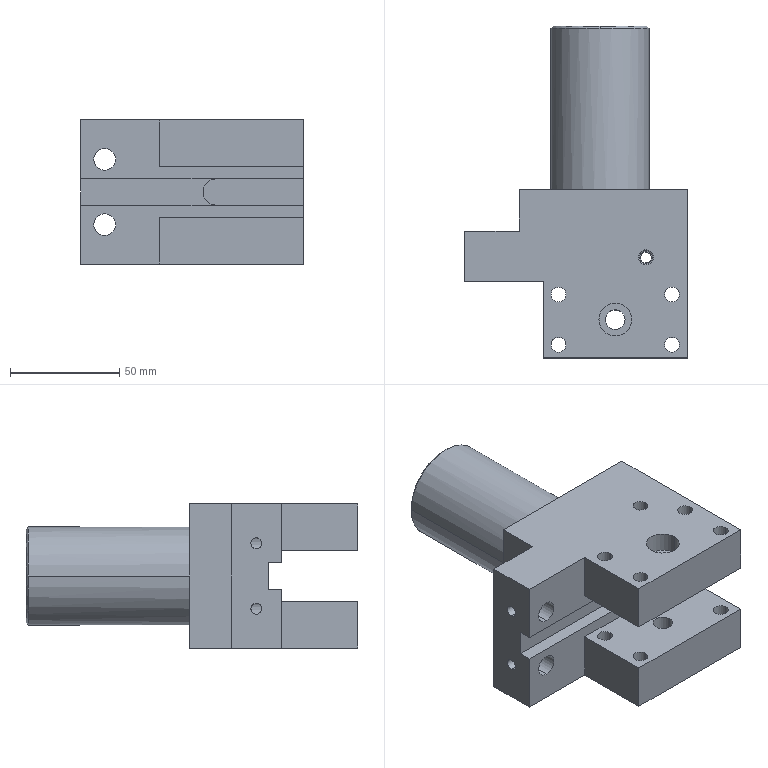Part | SolidWorks | features ICE 6, HoleWzd 5, Chamfer 1, Extrusion 1, MirrorPattern 1 | 1 solid | 74 faces | box 102 x 152 x 66 mm | volume 438428 mm3 | cylinder 45 | plane 23 | cone 6 | commonest cylinder face diameters 6.8 x18 5 x8 6 x4 9 x4 10 x4 15 x4